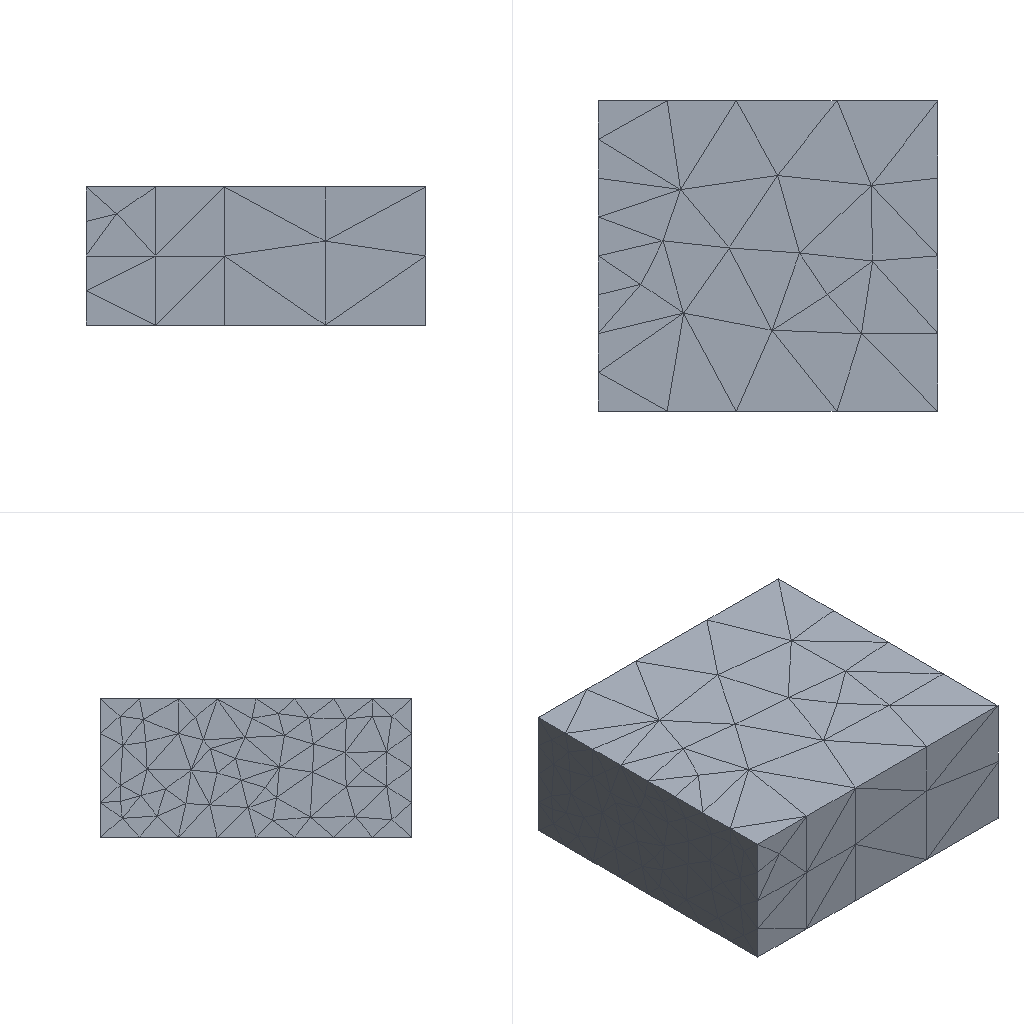Simulation study | ansys electronics desktop
Set-up summary:
category,name,step,type,value,unit,region
solver,ansys_electronics_desktop
units,length mm,,stated,model units
analysis,M06,,HFSS Modal Network,design_type=HFSS
setup,Setup1,M06,HfssDriven,frequency=10GHz; max_passes=2; max_delta_s=0.08
sweep,Sweep1_JEMY04,Setup1,Interpolating,8GHz..12GHz n=11 step=
sweep,Sweep1,Setup1,Interpolating,8GHz..12GHz n=11 step=
mesh,nodes,,,n/a (no mesh stored)
mesh,elements,,,n/a (no mesh stored)
material,vacuum,,permittivity,1
load,P1,M06,wave port,,,objects 34
bc,PerfE_TS6BF4,M06,perfect e,,,objects 58
bc,PerfE_YJ758H,M06,perfect e,,,objects 70
bc,PerfE_3KWRQP,M06,perfect e,,,objects 82
bc,PerfE_SXRUMP,M06,perfect e,,,objects 94
bc,PerfE_P8L5D8,M06,perfect e,,,objects 46
Ansys Electronics Desktop project file, long lists of numbers shortened, first 527 of 3724 lines:
$begin 'AnsoftProject'
	Created='Wed Sep 30 18:28:40 2026'
	Product='ElectronicsDesktop'
	FileOwnedByWorkbench=false
	$begin 'Desktop'
		Version(2026, 1)
		InfrastructureVersion(1, 0)
		$begin 'FactoryHeader'
			$begin 'geometry3deditor'
				KernelVersion(2, 0)
				ProjectContainsGeometry3D='1'
			$end 'geometry3deditor'
		$end 'FactoryHeader'
	$end 'Desktop'
	UsesAdvancedFeatures=false
	PreviewImageDesignId=1
	NextUniqueID=0
	MoveBackwards=false
	$begin 'HFSSEnvironment'
		Version(1, 0)
	$end 'HFSSEnvironment'
	$begin 'PlanarEMEnvironment'
		Version(1, 0)
	$end 'PlanarEMEnvironment'
	$begin 'Q3DEnvironment'
		Version(1, 0)
	$end 'Q3DEnvironment'
	$begin '2DExtractorEnvironment'
		Version(1, 0)
	$end '2DExtractorEnvironment'
	$begin 'NexximEnvironment'
		Version(1, 0)
	$end 'NexximEnvironment'
	$begin 'NexximNetlistEnvironment'
		Version(1, 0)
	$end 'NexximNetlistEnvironment'
	$begin 'EmitEnvironment'
		Version(1, 0)
	$end 'EmitEnvironment'
	$begin 'Maxwell3DEnvironment'
		Version(1, 0)
	$end 'Maxwell3DEnvironment'
	$begin 'Maxwell2DEnvironment'
		Version(1, 0)
	$end 'Maxwell2DEnvironment'
	$begin 'RMxprtEnvironment'
		Version(1, 0)
	$end 'RMxprtEnvironment'
	$begin 'MaxCirEnvironment'
		Version(1, 0)
	$end 'MaxCirEnvironment'
	$begin 'SimplorerEnvironment'
		Version(1, 0)
	$end 'SimplorerEnvironment'
	$begin 'IcepakEnvironment'
		Version(1, 0)
	$end 'IcepakEnvironment'
	$begin 'IcepakFEAEnvironment'
		Version(1, 0)
	$end 'IcepakFEAEnvironment'
	$begin 'SchematicEnvironment'
		Version(1, 0)
	$end 'SchematicEnvironment'
	$begin 'geometry3deditor'
		Version(1, 0)
	$end 'geometry3deditor'
	ReadVersion=12
	$begin 'DesignMgrEnvironment'
		CompInstCounter=1
		GPortCounter=0
		NetCounter=0
		Alias('Ieee;Simplorer Elements\\Ieee', 'Std;Simplorer Elements\\Std', 'Basic_VHDLAMS;Simplorer Elements\\Basic Elements VHDLAMS\\Basic Elements VHDLAMS', 'Digital_Elements;Simplorer Elements\\Digital Elements\\Digital Elements', 'Transformations;Simplorer Elements\\Tools\\Transformations\\Transformations', 'HEV_VHDLAMS;Simplorer Elements\\HEV VHDLAMS\\HEV VHDLAMS', 'automotive_vda;Simplorer Elem
	$end 'DesignMgrEnvironment'
	$begin 'ProjectDatasets'
		NextUniqueID=0
		MoveBackwards=false
		DatasetType='ProjectDatasetType'
		$begin 'DatasetDefinitions'
		$end 'DatasetDefinitions'
	$end 'ProjectDatasets'
	VariableOrders[0:]
	$begin 'Definitions'
		$begin 'Materials'
			$begin 'vacuum'
				CoordinateSystemType='Cartesian'
				BulkOrSurfaceType=1
				$begin 'PhysicsTypes'
					set('Electromagnetic')
				$end 'PhysicsTypes'
				$begin 'AttachedData'
					$begin 'MatAppearanceData'
						property_data='appearance_data'
						Red=230
						Green=230
						Blue=230
						Transparency=0.95
					$end 'MatAppearanceData'
				$end 'AttachedData'
				permittivity='1'
				ModTime=1499970477
				Library='Materials'
				LibLocation='SysLibrary'
				ModSinceLib=false
			$end 'vacuum'
		$end 'Materials'
		$begin 'SurfaceMaterials'
		$end 'SurfaceMaterials'
		$begin 'Scripts'
		$end 'Scripts'
		$begin 'AnsysComponents'
			NextUniqueID=0
			MoveBackwards=false
			$begin 'AnsysComponentDefinitions'
			$end 'AnsysComponentDefinitions'
		$end 'AnsysComponents'
		$begin 'Symbols'
			$begin 'M06'
				ModTime=1790764121
				Library=''
				ModSinceLib=false
				LibLocation='Project'
				HighestLevel=1
				Normalize=true
				InitialLevels(0, 1)
				$begin 'Graphics'
					Rect(0, 0, 0, 0, 0.00254, 0.00254, 0.00508, 0.00508, 0, 0, 0)
					Rect(0, 1, 0, 0, 0.0004233, 0.00254, 0.0004233, 0.0004233, 0, 0, 0)
				$end 'Graphics'
			$end 'M06'
		$end 'Symbols'
		$begin 'DefInfo'
			M06(1002, 0, 0, 0, '', 1790764121, '', 'M06', '', '', '', '', '', 'Design.bmp', '', 'Project', '', '', 1790764121, '', 0, 0)
		$end 'DefInfo'
		$begin 'Compdefs'
			$begin 'M06'
				Library=''
				CircuitEnv=0
				Refbase='U'
				NumParts=1
				ModSinceLib=true
				$begin 'Properties'
					TextProp('Representation', 'SRD', '', 'M06')
					TextProp('Owner', 'SRD', '', 'HFSS')
				$end 'Properties'
				CompExtID=6
				$begin 'Parameters'
					ButtonProp('CosimDefinition', 'D', '', 'Edit', 'Edit', 40501, ButtonPropClientData())
					MenuProp('CoSimulator', 'D', '', 'DefaultNetlist', 0)
				$end 'Parameters'
				$begin 'CosimDefinitions'
					$begin 'CosimDefinition'
						CosimulatorType=4
						CosimDefName='DefaultNetlist'
						IsDefinition=true
						Connect=true
						Data()
						GRef()
					$end 'CosimDefinition'
					DefaultCosim='DefaultNetlist'
				$end 'CosimDefinitions'
			$end 'M06'
		$end 'Compdefs'
	$end 'Definitions'
	DesignIDServer=2
	MoveBackwards=false
	$begin 'HFSSModel'
		RepRewriteV2=true
		Name='M06'
		DesignID=0
		'Use Advanced DC Extrapolation'=false
		'Use Power S'=false
		'Export FRTM After Simulation'=false
		'Export Rays After Simulation'=false
		'Export After Simulation'=false
		'Allow Material Override'=false
		'Calculate Lossy Dielectrics'=false
		'Perform Minimal validation'=false
		$begin 'TemperatureSettings'
			IncludeTemperatureDependence=false
			EnableFeedback=false
			Temperatures(6, '22cel', 34, '22cel', 46, '22cel', 58, '22cel', 70, '22cel', 82, '22cel', 94, '22cel')
		$end 'TemperatureSettings'
		ObjsEnabledForDeformation()
		'Port Validation Settings'='Standard'
		'Save Adaptive support files'=false
		SolutionType='HFSS Modal Network'
		$begin 'DrivenOptions'
			AutoOpen=false
		$end 'DrivenOptions'
		HasTransientSetups=false
		MaterialDensity=1
		MassOfTissue=1
		VoxelSize=1
		TissueObjectList=-1
		AverageSarMethod=0
		UseAutoDCThickness=true
		HaveZwaveSupport=true
		SolveInsideThreshold=100000
		RequireBodyFaceInfo=false
		$begin 'OutputVariable'
			NextUniqueID=0
			MoveBackwards=false
		$end 'OutputVariable'
		$begin 'ModelSetup'
			$begin 'DesignDatasets'
				NextUniqueID=0
				MoveBackwards=false
				DatasetType='DesignDatasetType'
				$begin 'DatasetDefinitions'
				$end 'DatasetDefinitions'
			$end 'DesignDatasets'
			VariableOrders[0:]
			$begin 'Editor3D Doc Preferences'
				BackgroundColorVersion=1
				'Plane Background'=0
				'Need Lights'=true
				'Ambient Light'=8355711
				'Num Lights'=1
				Light0[4: 16777215, 0.75, -0.15, -0.63]
				Ver=2
			$end 'Editor3D Doc Preferences'
			SnapMode=31
			WorkingCS=1
			$begin 'GeometryCore'
				BlockVersionID=3
				DataVersion=2
				NativeKernel='PARASOLID'
				NativeKernelVersionID=26
				Units='mm'
				ModelExtents=10000
				InstanceID=-1
				$begin 'ValidationOptions'
					EntityCheckLevel='Strict'
					IgnoreUnclassifiedObjects=false
					SkipIntersectionChecks=false
				$end 'ValidationOptions'
				ContainsGeomLinkUDM=false
				$begin 'GeometryOperations'
					BlockVersionID=2
					$begin 'AnsoftRangedIDServerManager'
						$begin 'AnsoftRangedIDServer'
							IDServerObjectTypeID=0
							IDServerRangeMin=0
							IDServerRangeMax=2146483647
							NextUniqueID=105
							MoveBackwards=false
						$end 'AnsoftRangedIDServer'
						$begin 'AnsoftRangedIDServer'
							IDServerObjectTypeID=1
							IDServerRangeMin=2146483648
							IDServerRangeMax=2146485547
							NextUniqueID=2146483654
							MoveBackwards=false
						$end 'AnsoftRangedIDServer'
					$end 'AnsoftRangedIDServerManager'
					StartBackGroundFaceID=2146483648
					$begin 'CoordinateSystems'
					$end 'CoordinateSystems'
					$begin 'OperandCSs'
					$end 'OperandCSs'
					$begin 'SubModelDefinitions'
					$end 'SubModelDefinitions'
					$begin 'Groups'
					$end 'Groups'
					$begin 'UserDefinedModels'
					$end 'UserDefinedModels'
					$begin 'OperandUserDefinedModels'
					$end 'OperandUserDefinedModels'
					$begin 'ToplevelParts'
						$begin 'GeometryPart'
							$begin 'Attributes'
								Name='Cav'
								Flags=''
								Color='(230 230 230)'
								Transparency=0.8
								PartCoordinateSystem=1
								UDMId=-1
								GroupId=-1
								MaterialValue='"vacuum"'
								SurfaceMaterialValue='""'
								SolveInside=true
								ShellElement=false
								ShellElementThickness='0mm'
								ReferenceTemperature='20cel'
								IsMaterialEditable=true
								IsSurfaceMaterialEditable=true
								UseMaterialAppearance=false
								IsLightweight=false
								IsAlwaysHidden=false
							$end 'Attributes'
							$begin 'PhysicsAttributes'
								SuppressedForPhysics='False'
								SuppressedForPhysicsEditable=true
							$end 'PhysicsAttributes'
							$begin 'Operations'
								$begin 'Operation'
									OperationType='Box'
									ID=5
									ReferenceCoordSystemID=1
									$begin 'BoxParameters'
										KernelVersion=23
										XPosition='0mm'
										YPosition='0mm'
										ZPosition='0mm'
										XSize='25mm'
										YSize='22.86mm'
										ZSize='10.16mm'
									$end 'BoxParameters'
									ParentPartID=6
									ReferenceUDMID=-1
									IsSuppressed=false
									$begin 'OperationIdentity'
										$begin 'Topology'
											NumLumps=1
											NumShells=1
											NumFaces=6
											NumWires=0
											NumLoops=6
											NumCoedges=24
											NumEdges=12
											NumVertices=8
										$end 'Topology'
										BodyID=6
										StartFaceID=7
										StartEdgeID=13
										StartVertexID=25
										NumNewFaces=6
										NumNewEdges=12
										NumNewVertices=8
										FaceNameAndIDMap()
										EdgeNameAndIDMap()
										VertexNameAndIDMap()
									$end 'OperationIdentity'
								$end 'Operation'
							$end 'Operations'
							$begin 'SubregionDependencyInformation'
								ChildSubregions[0:]
							$end 'SubregionDependencyInformation'
						$end 'GeometryPart'
						$begin 'GeometryPart'
							$begin 'Attributes'
								Name='Port1'
								Flags=''
								Color='(230 230 230)'
								Transparency=0.8
								PartCoordinateSystem=1
								UDMId=-1
								GroupId=-1
								MaterialValue='"vacuum"'
								SurfaceMaterialValue='""'
								SolveInside=true
								ShellElement=false
								ShellElementThickness='0mm'
								ReferenceTemperature='20cel'
								IsMaterialEditable=true
								IsSurfaceMaterialEditable=true
								UseMaterialAppearance=false
								IsLightweight=false
								IsAlwaysHidden=false
							$end 'Attributes'
							$begin 'PhysicsAttributes'
								SuppressedForPhysics='False'
								SuppressedForPhysicsEditable=true
							$end 'PhysicsAttributes'
							$begin 'Operations'
								$begin 'Operation'
									OperationType='Rectangle'
									ID=33
									ReferenceCoordSystemID=1
									$begin 'RectangleParameters'
										KernelVersion=23
										XStart='0mm'
										YStart='0mm'
										ZStart='0mm'
										Width='22.86mm'
										Height='10.16mm'
										WhichAxis='X'
									$end 'RectangleParameters'
									ParentPartID=34
									ReferenceUDMID=-1
									IsSuppressed=false
									$begin 'OperationIdentity'
										$begin 'Topology'
											NumLumps=1
											NumShells=1
											NumFaces=0
											NumWires=1
											NumLoops=0
											NumCoedges=0
											NumEdges=4
											NumVertices=4
										$end 'Topology'
										BodyID=34
										StartFaceID=-1
										StartEdgeID=35
										StartVertexID=39
										NumNewFaces=0
										NumNewEdges=4
										NumNewVertices=4
										FaceNameAndIDMap()
										EdgeNameAndIDMap()
										VertexNameAndIDMap()
									$end 'OperationIdentity'
								$end 'Operation'
								$begin 'Operation'
									OperationType='CoverLines'
									ID=43
									$begin 'LocalOperationParameters'
										KernelVersion=23
										LocalOpPart=34
									$end 'LocalOperationParameters'
									ParentPartID=34
									ReferenceUDMID=-1
									IsSuppressed=false
									$begin 'OperationIdentity'
										$begin 'Topology'
											NumLumps=1
											NumShells=1
											NumFaces=1
											NumWires=0
											NumLoops=1
											NumCoedges=4
											NumEdges=4
											NumVertices=4
										$end 'Topology'
										BodyID=-1
										StartFaceID=44
										StartEdgeID=-1
										StartVertexID=-1
										NumNewFaces=1
										NumNewEdges=0
										NumNewVertices=0
										FaceNameAndIDMap()
										EdgeNameAndIDMap()
										VertexNameAndIDMap()
										$begin 'GeomTopolBasedOperationIdentityHelper'
											$begin 'NewFaces'
												$begin 'Face'
													NormalizedSerialNum=0
													ID=44
													$begin 'FaceGeomTopol'
														FaceTopol(1, 4, 4, 4)
														$begin 'FaceGeometry'
															Area=232.258
															FcUVMid(1.51681195174844e-15, 11.43, 5.08)
															$begin 'FcTolVts'
																TolVt(0, 0, 0, 5e-07)
																TolVt(1.39977129142543e-15, 22.86, 5.07593966858622e-15, 5e-07)
																TolVt(3.03362390349689e-15, 22.86, 10.16, 5e-07)
																TolVt(1.63385261207146e-15, -2.25597318603832e-15, 10.16, 5e-07)
															$end 'FcTolVts'
														$end 'FaceGeometry'
													$end 'FaceGeomTopol'
												$end 'Face'
											$end 'NewFaces'
											$begin 'NewEdges'
											$end 'NewEdges'
											$begin 'NewVertices'
											$end 'NewVertices'
										$end 'GeomTopolBasedOperationIdentityHelper'
									$end 'OperationIdentity'
									ParentOperationID=33
								$end 'Operation'
							$end 'Operations'
							$begin 'SubregionDependencyInformation'
								ChildSubregions[0:]
							$end 'SubregionDependencyInformation'
						$end 'GeometryPart'
						$begin 'GeometryPart'
							$begin 'Attributes'
								Name='Short'
								Flags=''
								Color='(230 230 230)'
								Transparency=0.8
								PartCoordinateSystem=1
								UDMId=-1
								GroupId=-1
								MaterialValue='"vacuum"'
								SurfaceMaterialValue='""'
								SolveInside=true
								ShellElement=false
								ShellElementThickness='0mm'
								ReferenceTemperature='20cel'
								IsMaterialEditable=true
								IsSurfaceMaterialEditable=true
								UseMaterialAppearance=false
								IsLightweight=false
								IsAlwaysHidden=false
							$end 'Attributes'
							$begin 'PhysicsAttributes'
								SuppressedForPhysics='False'
								SuppressedForPhysicsEditable=true
							$end 'PhysicsAttributes'
							$begin 'Operations'
								$begin 'Operation'
									OperationType='Rectangle'
									ID=45
									ReferenceCoordSystemID=1
									$begin 'RectangleParameters'
										KernelVersion=23
										XStart='25mm'
										YStart='0mm'
										ZStart='0mm'
										Width='22.86mm'
										Height='10.16mm'
										WhichAxis='X'
									$end 'RectangleParameters'
									ParentPartID=46
									ReferenceUDMID=-1
									IsSuppressed=false
									$begin 'OperationIdentity'
										$begin 'Topology'
											NumLumps=1
											NumShells=1
											NumFaces=0
											NumWires=1
											NumLoops=0
											NumCoedges=0
											NumEdges=4
											NumVertices=4
										$end 'Topology'
										BodyID=46
										StartFaceID=-1
										StartEdgeID=47
										StartVertexID=51
										NumNewFaces=0
										NumNewEdges=4
Last 209 lines:
3eHl6goOEhYaHiImKkpOUlZaXmJmaoqOkpaanqKmqsrO0tba3uLm6wsPExcbHyMnK0tPU1dbX2Nna4u\
Pk5ebn6Onq8vP09fb3+Pn6/9oADAMBAAIRAxEAPwD+/iiiigAooooAKKKKACiis7WNY0jw7pGq+IPEG\
q6boWg6Fpt9rGt63rF9a6ZpGj6RplrLe6lquq6leypDp+m29nBNNPPM6RRRQtJIyopIANGiviP9mX4v\
/E74pfGL44y+MrnUtJ8D3/w8/Z/+JPwu+F+t6DpWleIvhXpHju5+Mfh/UtE8U39vpNve33i6/X4caRq\
urWd5LdRaFqWr3WhafdXtpp66pqP25QAUUUUAFFFFABRRRQAUV/Lb+0J/wXq+Mnwp/be8d+APCXwv+F\
+vfsRfBn9oL4cfAf4u/F+88O+OL7xtpOqa2mpweN5LDxFpvj6DR7fUIr3wZ8Tn0iGTSLhLq28Eu0jkz\
Ap/Ttrfijw14a8Nav408R+ItC0DwdoGhX/ijXvFmt6tYaV4a0Tw1pVhLquqeItX12/uI7XTdCttLgnu\
bi7mlS3ht4XmkkWNSwANyivna6/a/wD2S7LQPCHiu9/ai/Z2tPC/xBN8PAXiS6+Nnw1t9A8bnS9YvfD\
2pjwhrEviYW/iU2+v6dqFjP8AYpJvJvLCa2k2zROi+63uuaJpujXHiPUdY0qw8PWenvq93r17qFpa6N\
a6VHAbqTU7jVJ5lgg09bYGRpmkEYjG8tt5oA1KK8L+Hv7UP7M/xb8QzeEvhT+0T8C/ib4rt455Z/DPw\
9+LfgDxp4hgitVZ7qSbRfDfiC5uY440VjIWiAQKSxAFdd4L+MPwj+JGveOfCvw7+KXw58e+J/hjrJ8O\
/Erw54L8b+GfFOvfD3xALzVNPOheOdH0PU57jwnrP2/Q9ag+y38dvP52j3UWzfbyqgB6NRXnOpfGH4S\
aN8SfD3wa1j4pfDnSfi/4t0m41/wp8KdS8b+GbH4k+J9Cs4dYubvWvD3ga61NNU1rSYrfw74gkkuba1\
lhRNCvHZwtrOU4LU/2tv2VNF8Zv8ONZ/aa/Z80n4hRX50uXwHqfxn+HFh4zj1MS+QdOfwvdeJEvkv/A\
Dvk8kwCTd8u3PFAH0HRR16UUAFFFFABRRRQAUUUUAFfFXx98Vt8R/F7/A3SpZD4O8Lx6Pr3xzmWWK40\
nxfaeItI8Qr4f+BF0LLLpJKP7A8S+KrS4uLXfoFz4e0e803XPD/jnUhZfQPxi+KFt8J/B668ul/8JH4\
i1nXNE8IeCPCUeox6bceKPF3iO8W0sbQ3Itrme30OxsV1LWteu7Sx1G60rw34X1nWU069TTpLd/kbwX\
4au/DWirHresyeK/GeryQ6z8QPHN1aCx1Hx542m0+xstZ8VX9oLmYadHKlhawWOnRStZaLpWn2Gh6Wl\
vpOm2NrAAdb+z1/ycl8fP8Ash/7Mf8A6nv7WFfcFfD/AOz1/wAnJfHz/sh/7Mf/AKnv7WFfcFABRRRQ\
AUUUUAFfIX7ev7TFj+yB+yF8dv2gZ5rdNX8D+CL5PBVtchHj1H4ieIpIfDXgCweB8m4t38W6vpDXKqr\
FLSKeUqUjYj69r84P+Ckf7AWpf8FD/Afwq+FGofG25+E/wz8HfE6x+IvxC8P6f4EfxXqPxMi0q0k03S\
9Ah1tfHGkjwnDDYap4jPnNbaorXOoWl19nD2CLMAfxofCb9tf9h7QP+CW/x4/Y/wDiZ4K/aA8Q/tJ/H\
PxZr/xb1b4n6f4R+HmqeErP4raLqdndfC1/+En1b4r22sSeH0tNCsk1af8Ask3EZ8Y68Le2uxKpuP6H\
/wBk/wDan/4al/4IBftD3mr6l9v8e/Bf9jz9pr4FePTLL5l3Jd+AvgX4mi8Japcs58y4kvfh9e+FJpr\
hx++vfto3u0bmv6IdM0zT9F03T9H0myttO0rSbG00zTNPs4kgtLDT7C3jtbKytYIwFhtoraKNERQAqx\
gAYFfj/wDDz/gkt/wqvVP+Ckem+Bvj/wD2T8Jv+ChPgT4leHv+FXt8KvOg+C3i74haP4t0mPxdo2tp8\
SI4/FGm2K+O/E4GlJp+j/abc2Fs1/ELBJJAD8Jf2XP+CV37L/xT/wCCJfxH/bI+IGm+Ldf+O9t8Gf2m\
fib4A8Snxr4kstN+H0HwO134nJo3hbRfCtlqCaXeaLf6n4G1C5v/ALdaXUzSeJ7p7aW2k2SL9QeHf2f\
P2nf26v8Ag3T/AGZPh78Dtaude+IuleJ9e1HU/Cd/4jt9Fm+JPw4+F3xk+NXg3SPh3Fq2s3kFmi2UNr\
4LvbOC9uILU/8ACDW8CyI4gFfqx4S/Zs+Cv7Hn/BNyP/gnB8WP2u/hd4TvfiF8J/2h/g94X+KnxEfwn\
8MrrW7r46az8Rr99V0H4b+JfiUX1640iX4lwRGyt9aZr1tNQm4szdBYfPof+Cff7I3hL9gX4T/8En/2\
j/2j/A+v6/JdeJta+GHiCbWPB/wm+KWs+LvEXxQ8deO/D/ij4c/DrXvGGrT3t9ZTeMdQ0loopdRi1C3\
S7jdYhdNDCAfgPN8X/gP4K+IX7OXhf9u3/gnX8Tf+CafxO+FPxB8O6j4R/ah/Y68MaN8H/wC1tV014L\
ZLvxZoPj3wBqVv438IQ3cdtfX1/Z6vrmohLSVbQvDLdWt5+qPxN1GD/gnT/wAF0PBnxKup4vD37Pf/A\
AUm8Fjwj4vuriRLLw/pHxj0y40zSv7ScyssUd3/AMJhB4Iurq7mkVYovi3qspwqkHvJf+Cd+lfGn4rf\
Cj9nT9sn/grHb/tZ6H8C/EekeOPCv7IE/h34MfDv4kX154X0eePSpviLPonjPUPE3jS1Xw7d3kd5c3l\
kt7NY6jdGO9tTcSTV8Cf8F2f28v2O/wBrL4Tan+zn8OtUvPiB+0N8Jv2lfDNh8KbzwLpOva5pfiLw9f\
eAdIXxXr9t4kl8O29jfaFf+IfE2qaJZ2OkXmqy6ne+C9N1m3kbTbuBgAe/fsOeE/Gn/BST9qX/AIKc/\
t8+GvEM/hiK88C/ED9j/wDYw8bXBu4rfwZeal4LudF03x/pbQIZtI1Ow0IeENTm8jewn+JuqBAXAJ/K\
hfh34x/Ym+Bni79m/wD4KF/8ElIPGHw/urjX0uv2z/hJo+lwfGnwyusatcala+JdL+Pi+H/Emiale2U\
k0Q0zT7u50a3a0t4rXVbO5Auo5v6jv2Vfh3+zB/wT1/YH+Bf7L/7UnxO+CHwpn+IHw38Rn4i6L8Y/iP\
4J8A23xC8XeNbO31L4y6LaSeKtcsv+EostOl8Z2mjzPblzDYLp6S+UJYQfjfw1/wAEs9Rs/wBnvx18P\
P2cP+Cs3iDwt/wTi8dWfjrVNc8C2fgv4PfFDw9YfD7W5NRn+IWk6J+0dL4qj/sLwmYP7ZXUJIIo7bD3\
cuoLPLLeSTAH6tf8E7vFHwq8ZfsUfs7678EPHPxR+I3wpfwINK8F+KfjVc6LefFRtL8Oa1q3hyTw942\
uvDumWljPrOi32k3eilrWFojH4fj23F5zdzlen/sqfCT4OfAv9nP4O/C39n2+s9Y+DPhnwRpUnw+8RW\
GuWHie08W6F4gWTxMPG0XiTST9k1863d6zdas17ZhbO5fWWmtES3eNFKAPoGiiigAooooAKKKKAPg74\
rX13r/7T+p+HtYnkv8AQvhx8GfhZ418FaTMR9g0Lxh8SPFnx/8ACni/xRDbIAt14gn8L+B9D063u7gT\
T6bY3OqWumPZwa7riajo1h+P/wDk7f4lf9m5/s5f+rM/aurcoAP2ev8Ak5L4+f8AZD/2Y/8A1Pf2sK+\
4K+H/ANnr/k5L4+f9kP8A2Y//AFPf2sK+4KACiiigAooooAKKKKACiiigD8cv+Cp+p6T4w/4Rz9k/4M\
fCPwD49/bR/bK+HnjD4J6T481rwpo15qnwY/Zjv50X4u/EPxZ4x/s9tQ0fwTZ/2jJ/ZtilxFHd65MLm\
0iur6yW0ufxc/bJ+H3/AAqS1/4Ky/CuXWrzxL8Rfhn8Pf8Agiv8P/2afEfiQwt478QQ+DJ/B3hvVtb8\
OsSZW1K78RaZq09+bMkG6nm3EnNf1d/FH9lz9mb44a5ZeJ/jT+zr8Cvi/wCJdN0mLQdO8Q/FH4R/D/x\
/rmn6HBeXuoQaLZat4s8P3dxa6Sl/qWozpbRyLCs1/PKEDyyM2V40+E37LHgKx8JfE/xj8HfgxpX/AA\
o7QNA8NfDXxM/wp8KX/iD4c6Jps9po/gzwV8KU07w3NqOkyHUbjTdP0LQ9AjFxc3t7a6dpVlLdzwQOA\
fiB+1ZdeHf2pv2/fh9+y1+zL4C0j4e+Bv2XPj1pn7U37Zn7QPwz0O38Fa3qnxum8L6vZ6X4Gj8aeDrr\
Sb2fxlqmj382nazqsWoS635+pmeJCfC14T4j+zn4D/Z+/wCHwfwQ8Q/Crwr8DvEvwsv/ABB+0tb/AAr\
H7Pfh/wAA6VYeAPGfgX9lz9nK78VeLviVrHhCyubbxn4LbVfEGuaboFnG2nroXi++1S9VpL6e8WX9Kv\
A37LPwQ1DX7n45/EL9nD4I2/x88c+P9Q+NniHxBc/DL4bap4t8EeONc1pPEWj6RpnjHTtEIn1zw5BDo\
tg+vacbSTXNV0G58V3CDWNYv7iX6P8A2LPhd8M/C/jv9rjxj4Z+HXgTw74u1X4+afpOqeKtC8I+H9I8\
R6lpVx+zz+zz4mn0y/1zT9PjurzT38Savq2oPDJK0bX2qXF2ym4nlkYA+R/+Ciep/EPRv+Clf/BH/U/\
hT4P8LePvH9nb/wDBQ2Xw94P8aeOtQ+GvhzXJP+Ge/Bq39rfeNtL8DeJJtEnXSWv5bU/2NdRXF3BBaz\
y2ME8t/a/E/wAO/g74I+Mn/BIX/gojrvjzV/EWk+OtH+M/7f37TfxN+BPh3WtY8I6Z8D/jzo/wz8dQ6\
f8AAfxZZ6dcRf8ACX+C9A1NdA8SWtuVh02+1SDTb17d0tXgk/pe1n4e+AfEfizwX498Q+B/B+veOvhv\
/wAJH/wrvxprPhnRdU8WeAv+Ew02LRvFv/CF+I76ykvPC39qaPBBaaj9hmg+3W0KQXPmxKEGFH8Ffg3\
CvxOSH4S/DKJPjZFcW/xmSPwH4VRfi5BeaXeaJdw/E5V0oDx7FLouoX9pIuq/aw9rfTW7AxSujAHhv/\
BPb/kwX9h7/s0D9mn/ANUx4Kor6n8PeHtA8I6BofhTwpoej+GPC3hjR9M8PeGvDXh7TLLRdA8PaBotl\
BpujaHoejabBFb6To9pp1tbW9tbW8ccMENukUSJGiqCgDYooooAKKKKACiiigD4D8f/APJ2/wASv+zc\
/wBnL/1Zn7V1blYfj/8A5O3+JX/Zuf7OX/qzP2rq3KAD9nr/AJOS+Pn/AGQ/9mP/ANT39rCvuCvh/wD\
Z6/5OS+Pn/ZD/ANmP/wBT39rCvuCgAooooAKKKKACiiigAooooAK+HPjjrd34z+Oun/C+/eRfBnwz+H\
ng34s6hobyCbTvGXjbx1428Y6V4A1TVLdEjKx+En+DviK9s7a4e9srvVfG+n6x9ls9W8KaPen7jr4D8\
f8A/J2/xK/7Nz/Zy/8AVmftXUAblbn7JP8AyGP2qf8As4zSf/WXf2aaw63P2Sf+Qx+1T/2cZpP/AKy7\
+zTQB9iUUUUAFFFFABRRRQAUUUUAFFFFAHwH4/8A+Tt/iV/2bn+zl/6sz9q6tysPx/8A8nb/ABK/7Nz\
/AGcv/VmftXVx3xU8b6h4N0XRrbw9BY3njPxt4o0vwV4MtdTjuZdNXVb+C+1jWta1GK3uLcXljovgjQ\
/FmvTWTXunvqsfhdtJtL+2v7+0egDB+GX7Qfwz+Hv7Tf7Qlp4gk8e3c1n8MP2c/Cl6fB3wd+MPxGhsf\
EGl6r8efGV5pt9dfDzwHqkVlKPDXxG8HXSNK6RzDVmiheSa1vI7f7N0L9qv9mjxHqWjaDpfx7+Eg8U6\
9fadpGneCNU8e+G9B+IA8QapcQ2Vp4V1H4f67qFtrWjeMf7RnjtJtGvLC31S3vd1lcWkV2jwr8IfBjw\
tYeCvFvibwvp1xfX0GkfDP4VQz6tq0sNzrmv6lN4m+Md3rHibxHfQW8Q1XxRqer3F9qGp3pjWS91DUr\
m7lBlmcn3/AFPTNN1vTdR0bWdOsdX0fV7G70zVtJ1O0t7/AE3U9Nv7eS0vtO1Gxu43ivbGa1lljmhkR\
o5I5WR1ZWIIB93UV+Xtl8A/hVofm/8ACEeHb74Tfatn9qf8KN8W+M/gP/b/AJG/7F/wlH/CmvEGhf8A\
CVfZfOu/sX9pfavsP9pXf2PyPtl153R23hz4naNAmm+E/wBpf47+GvD9tu+waJc3Pwp+JE9l5ztPdb/\
Gnxq+FPifxNrPmXstzMP7T1y++zicWln9m0+C0s7cA/R+ivg6z+LP7VOhStd3/wDwz78U4ZIzbL4fs9\
B+I3wDls5XZZV1lvGE3iv4kjUo40heA6Z/YVoZjqIuv7WgFmbO/wCjs/2o/iNpUTW/jP8AZn8Xanqjy\
Ga3n+CvxI+GPjjwslgyqkUN/q3xd1z4d6lb+IBcR3TS28GiXViltJaSxapPcTXNpYgH2dRXy9bftk/s\
+vOi6v4l8Y+CNPO77R4n+KPwZ+Nfwl8C6ZhGMX9ufEH4nfDzSND8P+dOIre2+3ahb/a7y7t7G2828ub\
eCX1vwB8YfhH8WP7W/wCFWfFL4c/Ev+wPsH9u/wDCAeN/DPjL+xf7V+2/2Z/a3/CO6nc/2b9p/s3UfI\
87Z532Cby93lPtAPRqKKKACvgPx/8A8nb/ABK/7Nz/AGcv/VmftXV9+V8B+P8A/k7f4lf9m5/s5f8Aq\
zP2rqANytz9kn/kMftU/wDZxmk/+su/s01h1ufsk/8AIY/ap/7OM0n/ANZd/ZpoA+xKKKKACiiigAoo\
ooAKKKKACiiigD4D8f8A/J2/xK/7Nz/Zy/8AVmftXV87+BL4/EbU5vjdd82ninRV0f4ZWGWmtNL+Fia\
zqOp6L4oszefvrHXPGNlJoOt6rGItPeOysPDeiajYNqHhyW/vN79p7Sdb8X/tc+KfAf2PyvAOvfs5/s\
/av8QNaS5t3lvrLwv8ZP2hbzTvhm+kzTr9q0XxN9r1GLWpZob2zl0HQdV0O4tFl161v7DtqAMfwT/yV\
Tx//wBk/wDhX/6kfxgr2ivF/BP/ACVTx/8A9k/+Ff8A6kfxgr2igAooooAKKKKACuH8Z/DH4bfEb+zf\
+FhfD3wP48/sb7Z/ZH/CZ+E9B8Uf2V/aP2X+0P7N/tzT5/sPn/YbLzvK2+b9ji37vLTHcUUAeV2vwk0\
nR/s7eEvG3xp8EtpXkt4ZsvDHx0+LsHhHwi1jtOjWvh74X6n4yuvCUPhywMVslpoFxoNx4dW2tI9Ol0\
ibTA1m3VWWr/tKeG/N/wCEf/aAsfGH23Z9r/4Xl8IfCPir+zvs+/7P/wAIv/wpG++G32DzvPm+2/2n/\
bPm/ZbT7F/Z3l3f27qqKAILb45/tOaTAmn3nw1+BHj+5t93meLrb4pfED4QQat5rtOmz4dS/Cfxw3h7\
yI5FtTnxRqn2s2Rvh9iFyNOtPlrxX+0ppD/tN+P/ABD4v+Fvxk+H1je/An4GaNFDqXhbRPiFqaXek/E\
D9o6+gluNJ+BHinxfcW9hew63ei2uHjEMUnhq8iv3sXuNIXVPqyvjPxr/AMnJeO/+yH/A/wD9T39oug\
D1O1/af+AMkZOr/FHw14GuQ5CaT8VJLz4Q+IbiDapXUbPw18UbTR9QvtGeQyxR30Ns9nLPaXFvHO09t\
cRxfSv7JP8AyGP2qf8As4zSf/WXf2aa+B/FvinTvBug3Wv6nHd3EMNzpenWtlYRxS3+qaxr2rWOgaBo\
9kLmeKCK7vdd1PTrWOW5nt7SF7xZbu5trZJZ4/oj/glzoE3hj4WfHHRbqz8Pade2/wC0G1zqOneEdKs\
NE8Kadqmp/AD4Aapqlh4a0zT9NtFg0CDUL25is2mhN7LbxRzahPdX0lzczAH6aUUUUAFFFFABRRRQAU\
UUUAFcR8RvH+i/DLwjf+L9dg1K9tre/wDD+iadpWjwW8+r6/4n8YeI9J8HeDfDGlC+u7a0t9S1Txdr2\
iadBPf3dlpttLqa3GpX1jYRXF3D29fIUeoD4u/Fy48dxM0/w5+EDeL/AIfeAYrgNENY+Llp4k1rwX8Z\
vG02jXTSiJdCHhv/AIRLw5qezTdSU6v8QoxDfeHdb0bUb0A+UNO8Iaz4S+JXiR/F9zp+pfEbxb8OPh5\
45+KGs6XNdXmnaj4/8T+NfjRea1a6LqGp20V9eeDNIhWx0Dwwmo+Ze2HhbwlomlSzSCwQ13lXviN/yX\
bxN/2SX4V/+pj8aqo0AY/gn/kqnj//ALJ/8K//AFI/jBXtFfNWiePvAnhn4sePofEnjXwl4fmPgf4Y2\
gi1vxHo+lSG7t9Y+KF/PbBL+8jJuEsdW0qZ0xuWLU7eRgEmjLfRlle2epWdpqOnXdtf6ff20F7Y31lP\
FdWd7Z3UST2t3aXUDslzbSQSI8ciMyOjhlJBBoAs0UUUAFFFFABRRRQAUUUUAFfGfjX/AJOS8d/9kP8\
Agf8A+p7+0XX2ZX5yfHzxRqWn/tJeJPCHhe6+yeMvF3wP+C1xZXzW9vLFoPhPQ/if8bLfxv4oV76KS3\
bVLXT9esrfS4ZIL5ZdY1rT3utPn0mHVJrYAwbq/wD+Fg+Mhq6nf4O+Huranp/hcbfstzqPxG0yTxX4I\
8da3cpzNLpOnWlzf6LpySG1Sa6n1y7ms722Xw9qSfon/wAE9f8AkWv2i/8As4xf/Wd/2ea+CdE0bTfD\
mi6R4e0a2+x6PoOl6fo2k2fnXFx9k03S7SKxsbb7RdyySz+XawRLvkd5G2bndmJJ+9v+Cev/ACLX7Rf\
/AGcYv/rO/wCzzQB+g1FFFABRRRQAUUUUAFFFc54x8W+H/APhHxT478W6h/ZPhXwV4c1zxb4m1X7Je3\
/9meH/AA5pl1rGs6h9h0y2mubzydNs7mTyreGWeTy9kUckhVSAeM/tB+JtUudL074L+DNV1LRviD8YN\
N1qCHXdKvLvRdQ8FfC7Q9V8J6P8X/iJo/iS2mR9G8ZaboPjbTLTww9ul9cr4q8UaHdz6bNoVnrt7p2z\
pOk6VoGlaZoWhaZp+i6Joun2Wk6No2k2Vtp2laTpWnW0dnp+maZp9nGkNhp8FpDDFDDEiRxRxKiKqqA\
PPfhtoXiA3njX4j+ObFtP8d/E3xFJql1pU91aahceDPAeiedpHwv+HUd3aXd3HZtp/hdBqWs2NnqWo6\
MnjXxt4u1HRbqSw1WNm9SoA+PfiN/yXbxN/wBkl+Ff/qY/GquT8Ra2dEsrd7e0/tHVdT1Gx0XRNKE5g\
bUNV1GYRRLJIkMskWnW1sLq+1CaGC5ktNN0u8vRbzLbNGes+I3/ACXbxN/2SX4V/wDqY/GquD8LQ/8A\
CU65d+MbhftGgaf5Fj8P9432d0rWU39uePNO5Tf9u/tKTTLKaSJ8WGiTXumXb6d4hm88A6vwr4eXw3o\
8FlNdDU9XnEd54i154Ps1z4j1+S2t4NQ1q6hM0n2cy/Z4kgt1kaGxtLe3sLQR2drbxR4938L/AIc3l5\
c6nL4G8Kxaxd3M1/Jr1loen6d4ij1OeVrh9XtPEWnwRX1hrQunM0d7BcR3UU4E8UyTKrju6KAOETwRd\
WGf+Ec8f/Efw75uPtm/xMPG/wBs8vP2fH/C1LHX/wCzPL3z/wDHh9k87z/9K8/yrfybCR/FTTNqWPjH\
wz4jsrU+bHB4t8IzWviLVgD50ljf+KfCuuWen6aZJC8MN1B4ak+ywGJ5bPUZopGuezooA5VPGvxCsT5\
us/DSwv7Vh5ccPgTx5Z67q63Bwyy3Np420HwzaR6aI0lDyR381wJXhVLSSN5ZrewnxX0y2Hl+IPCXxG\
8OXpO+KxfwRrHjAy2pwqXf9p/DGPXbCANKsyeRNdx3i+R5klskMtvLN0VFAEGj/E34beIdRt9H0D4g+\
B9c1a8877Jpej+LNB1PUbr7PBLdT/Z7Kyv3ln2W0E0j7VO2OFnbCqSO3rz7VtH0nXtPuNJ13S9O1rSr\
vyvtWmatZW2o6fc+RPHcwfaLO8ieObZcwwyJuU7XiVxhlBHIJ8L/AAZajy9GsdV8J2pO+TTvAnirxZ8\
P9ImuDhWvbnRvBOt2Fpc6k0axRvdSQtcPFbQxPK0cMSIAe4UV4uvhrxZZbTpPxU8ZxxWmDpml61YeCd\
f0mOOD/jzsNWurnwpHrWt6cFSOOeSTWk1S5iDs+qLdubsWU1X4u6bnzIvhx4z87GNjeJvhn/Zvl5znd\
/wlv9t+d5g/6B/2b7L/AMvX2j/RgD0PxP4k0Xwb4a8Q+L/El7/Zvh3wroereJNe1H7Pd3n2DRdDsLjU\
9UvfslhBLPdeVY2s7+XDFJK/l7Y43cqp/N+5v/GOr/Hb4ha143/0TU9Y+Gvwxv8ATfDqrpezwh4Xf4g\
/H+Hwr4bnm0oypda5HoMFjca1J9v1SA67qWqLpl++jLpsEHpvxK+LPiLxZ4qsfBerfDHxTf8Agv4ceI\
bPVfi7eeBr3w94js7fx34eb4d/E34Y2mmnUtT0zxF4m8OafpWq22v6rBo/h4andarpekaVp41a0Or6b\
f8AgniX4yfDt/jj4u1bU9Zv/CGmXPwo+FOnQX/xG8L+LPhjay31h4v+NVzNaJN8Q9D0wNcPb6nE9suc\
3i2d8bTzhp2ofZgD2KvuL/gnr/yLX7Rf/Zxi/wDrO/7PNfn/AOHvFPhjxdZS6l4U8R6D4n06C6exmv8\
Aw9q+n61ZQ3sUUE8lnLdabcSxx3SwXNs7Rlg4S4RiMOpP6Af8E9f+Ra/aL/7OMX/1nf8AZ5oA/Qaiii\
gAooooAKKKKACvkn9qvQNQ8Zaj+zJ4HtPF/iTwVaeK/wBosLqmq+GIPCt9fOvg/wCAnx4+JWgLJpPjr\
wxrWjamtt408EeF9Rtxf6VefY7/AESz1Ox+y6pY2F9a/W1fN/xz/wCSkfsf/wDZxnib/wBZJ/akoA5V\
/BX7VejqdRj8e/s+fEN7fG3we/wu+I/wbXWPOIgOfiQvxd8dnw59nEpuv+RU1X7YbL7B/oP2r+0rOjJ\
4w+PegMLPxP8Asza54mv5R9phv/gh8VPhd4v8KQ2bkxR2moal8adc+HGqQeIVmhuHlgt9DutPW2uLSS\
LVZ7iW6s7H64rH8QeINI8L6Re69r16thpdgsRnnMU9xLJLcTxWllZWVlaRST6lqlzfXFtbWlpbRy3V3\
dXUNtbQyzyxxsAfkN8ZPi1a33xf1K3vvDPxg8AWt14J+FmjfELV/EHwp+JWk2Pw60jQvE3xn1jxjca5\
460vw/Lodr4fKImkN4r0zXpNBt01S517SdfurPSJrpfVPAfj74X+MrSew+GPjTwD4rsPDVtptnc2XgP\
xH4e1208P2k0U8Oj2s9t4fvJU0q2eHTrlLZGWNWWxkWIERMF+gvD0er3i3XinxVC0fi/xSw1DWIJriC\
9l0Cxa5vLvQvAtte2jGCfS9DsdQayjktUht726W81hoFvdUvZJcfxt8LPhj8S/7M/4WN8OfAfj/wDsX\
7b/AGN/wm3hDw/4q/sn+0vsn9o/2Z/bunz/AGDz/sFj53lbPN+xRb93lptAOSorFm/Zj+FVuXk8JReM\
/hq8S+Zotj8NfiN478H+DfDN+i74dR0T4Uadr/8AwhysL8G8uLS68P3Wm6ldyzzatY6h9rvFuMub4J/\
E3SlFx4W/aF8R6tqDsIZrb4vfDz4c+LvDSWbAvJPY6b8KtG8BajBrgnjt1inm1i5slt5bmOTTZp5be6\
swDrqK4Gbwz+0rorC1gtPgb8SkkUXB12bXvH3wQa0ZyYzpI8KJ4Y+II1BYxEJv7R/tq1837ebb+y4fs\
n2u9ypPiB4z01GvfE/7Pvxt8NaHDj7drUdn8NPHz2XmERW2PCXwh+JviPxFq3mXklvCf7O0a88gT/ab\
v7PYw3N1AAep0V41N+0J8GdOYQeKfHuk/DjUHUSw6H8XoNT+DXiW6s2JSPVbHwx8VbHR9Rv9DedLiGK\
/htZLKW4sbm3jnae1uI4vWNN1LTta07T9Y0fULLVtI1aytdS0vVNNuoL/AE7UtOvoI7qx1DT761keK8\
spraWKSKWNmjkjkV0YqQSAXaKKKACvNfip42vPBnhuNNAhs7zx14tvLnwp8ONO1OG4k0a98az6DreuW\
UniGW3uYGtfDNlpeg6vqepsk6XT2GiXMGmpd6rNY2N16VXyp4e1P/hZfiAfF+U+ZoFzpE+lfBxQn2SV\
fht4ltfCms6p4l1azBaQav4h17QbC8hjuZS9noekaHE2n6NrEviG3uADo/DHhyz8K6OmkWc95eFr/Wt\
Z1HUdQe3a/wBY1/xNrWoeJPEuuXy2dtBbwXl94h1bVLyWG0t7ayge9aGytbW1SG3j+dvFf/JevGP/AG\
SL4Rf+pl8c6+qa+VvFf/JevGP/AGSL4Rf+pl8c6AOY8V+C/h5rs0Or+L/A/hnxTqKiw0XT5NS8H2Piv\
Xrya+1EWujeHdDs/wCy7m91XUrvWtTS3sNOs45bi7vdTS3tIJbm4SN/2U/Yw+At78Afg4mma9Lri+Nf\
iJrcfxQ8f6NrniGfxXJ4R8V614T8KeHpfBNl4kvNY1KfX7fSNG8K6NYTX8mo3UeoX1ld39iun6bdWWk\
6f8cfsjfBmX4q/EO2+Jmv2dx/wrX4S63bX3hWSWztLnRfiP8AFSxPiPSb2BxqO5bvRPBV/Fp18s9vbT\
I3jE2H2TVbDVPBer6fcfr3QAUUUUAFFFFABRRRQAV83/HP/kpH7H//AGcZ4m/9ZJ/akr6Qr5v+Of8Ay\
Uj9j/8A7OM8Tf8ArJP7UlAH0BXzL451v/hOPGaaRaT/AGvwP4Hy1/5T+bpXiP4kwaqNltJhE+1/8Ir/\
AGRuIDXlg2teI8MtvrnhX/R/R/iz4uvfDvh19I8N3iweO/FayaT4UEcdvdXWlCWazs9a8cPY3dvJBc6\
XoFjqK6hKl35VreXMVlo/2hLzVrKOXyvTNMstHsorCwiaK3iaeUmWe4u7q5uru4lvL6/v768lkn1LVL\
m+uLi4urq4klubq5uZbi4llmlkkYAv0UUUAFFFFABRRRQAV4rq/wCzf8ANb1HU9cvvgx8M08Tave3ur\
XnjHTfBmg6J44TXdQnlvLjxLp/jjRbK31fSPFY1CV7qLVbS9g1G3vAt5BdR3KJKvtVFAHzrN+zjpVjt\
/wCEI+K3xx8A+bn+0/J+ILfFL+1tmPsW7/hoXSfGf9heRvu8f2R/Zv2r7Yf7Q+2fZ7L7LmzfC746aIX\
Xw78W/BnjDS7BftFjp3xK+Glxa+MvEDKv2mbSdb+Ivw98W6ZpGiLPdma2t9Rs/Ak/9nWjwST6XrV1bz\
Pf/TlFAH50fFS8+MWr634Z+CnxA8HfDbw34W+KPhrx/qXjDUvB/wATvE3jPVL/AMAeFI/DWh+JfCdnb\
618INBXSb3VtT+IXhi1lvEmkmi0c6ybKWw1b+zL6D0erfx4/wCS9fBX/skX7Qn/AKmX7NdVKACvmLUP\
D/ibxv8AtSXnw+8D2gvvF3iz4Z/Be3gLWb6ha+GvDMXxG+MFp4w+ImuWSX1osvhvQNJ1NbyeKW+09dS\
u3sNAtL6HVta0xJvpHUNQsNJsL7VdVvrPTNL0yzudQ1LUtQuYbKw0+wsoXuby+vry5dY7Szit4pJJZZ\
GVI0jZnYKCa+rP2TPgs+j3WvfH/wAaeG5tC+I/xE0K08G6HpGs6Jb2Ou+DvhH4Y8UeJ9T8L29zLfw/2\
npmu+JX1eDX9asLhdNeyT+wtC1HR4dX8OXl/fgH038Lvhz4d+Efw98I/DbwqLl9E8IaLa6TDfaiLFta\
128UNPq/ijxJdadY20Op+LNW1ie/1PV70QRPf6nq13eyr5s7k97RRQAUUUUAFFFFABRRRQAV8yftB39\
jpXjr9kzVNUvbTTdM039oHxdf6jqN/cw2djYWNn+yJ+1PcXd7e3dw6x2tpFbxySSSSMqIkbMzBQTX03\
Xzv+0X8Eda+Nuj/D218P8Ai/RPB+qfD/4iN46il8S+ENY8b+Htftbn4dfEP4c6l4Z1vQdC8f8Ahq4ud\
LudM+IV486HUjbXEdm1le2l3ZXVxCwBwVpeX3irXdY8c6zDdxPfXd/p3gzTtRhmguPDngWCW1t7OOK0\
uYYZNOu9buNLi12/S4tbbUom1Sz0fU/N/sGyEO7XBT6b+1Ho0TalrXwS+GniDTbbb9p0j4WfHq+8Q+P\
LvzmEEP8AYWkfE/4PeCtCu/LuJYpbr7d4m0zy7OG4ltvtl4lvp93hXPxU1DQZBZ+O/gt+0J4K1eRBc2\
2lW3wf8UfF9LjTXLRQ6gfEv7OMPjTQ7F3uobyP7Ddapb6rELQXE+nxWlzY3F0AetUV5R4c+OvwZ8Wa/\
a+ENC+KHga78b3b3cH/AAr6fxJpmm/Eayv9Ntbi81fRtZ+HmqXEOtaD4gsILO+/tHTr2wt77Tn0+4iv\
re3lt5kT1egAooooAKKKKACiiigAooooA+Ovjx/yXr4K/wDZIv2hP/Uy/ZrqpVv48f8AJevgr/2SL9o\
T/wBTL9muuX8QanqdhZx23hzRJvFnjPW5pNH8CeCrO5FpqHjTxdLY3l5pnh20u2glXToXjsbqe+1CZP\
sWj6Zp99rOpyW+l6fe3MIB2Hw++G7/AB2+IEXgm4tppvhj4Rmsdd+LerRW1veadqWp6ZqXhjXvDPwNv\
49Q/wBFvofEelXVxd+JbUxakIvCds2l6lYWS+NdC1aL9Za8i+CHwksPgx4Eh8Kw6l/wkOuajq+seKvG\
ni2TTYdMuvFXi7xDeNd6hfvbJPPNBpFnZrp2kaJa3d5qN1pfh3w1pGjvqN6unJcP67QAUUUUAFFFFAB\
RRRQAUUUUAFFFFABRRRQBzni3wd4R8feH9Q8JeO/C3hzxr4V1b7J/avhnxboemeI/D+p/YL221Ox/tD\
RtYtZra88nUrOzuIvMjby57SOVMSRqw8Muv2Pf2cPk/wCEb+Glp8Lvvfbf+FFeIvGH7Pv9ufd+zf8AC\
U/8KP8AEPh//hLvsv7/AOw/2p9r+wf2hefYvs/227876WooA+TLr9lrUdMaZvh7+0B8ZvCtlaIZ/D3h\
HxNceCvix4Qtb9EE4g8Sa18RPB95468VeH7nVfNmvrdvHNrfC3vJbHR9V0W3jsBY8/c/C39qbQUF5Z+\
LPgB8VZZHFs3h658J/EX9n9LNHDSnWR4yi8XfEs6m8bQrB/Zn9hWgmGom6/taD7ELO/8AtOigD4Pn1T\
496NK2m61+zB428QalbbftOr/Cz4j/AAR8Q+A7vzlE8P8AYWr/ABP+IngrXbvy7eWKK6+3eGdM8u8hu\
Irb7ZZpb6hd4E/x8+HmnRNe+Jrf4l+ANEh2/bfF3xT+B3xt+E/gPSfMYRW39u/ED4lfD3StE0Dz7t7e\
2tftt/B9qvL23srbzbu5ghk/Q+igD4q8G+PvAvxF0yfW/h9418JeO9Gtb+XSrrV/BviPR/E+mW2pwW9\
rdzabPf6JeTxQ36Wl9ZStCziRY7yJyoWRCetr1Hx38Bvgb8UdXtvEHxN+DHwn+IuvWemw6Paa347+HX\
hDxdq9rpFvdXl7BpVtqXiDR7iaDTUvNQv5kgVxEst9NIqh5XLeZXX7IvwxtRNP4E8QfFz4WanG5/sO4\
8F/Fvxxf+GvCdq0gR9J8L/CH4hatrvgTTPD6aY01jZ6afCslhpNrJH/AGNbadcWlhcWgBHRWPdfs7/G\
DRtn/CE/tKXes/ad39p/8L1+Efgzx59m8nb9i/4Rb/hS178M/wCyt/m3f27+0v7b8/yrP7H/AGb5N19\
vwrrwj+1N4baaOXwl8GfinpmmIbq51/wz468VfC/xf4mtVQXl1ZeG/hR4n8H67pOmeIERpbKxh1L4iR\
2GoXFrFd3uq6Db3csOnAHzf8eP+S9fBX/skX7Qn/qZfs117N+yj8N38Z+I1+P2vW0y+HdEh1fQvgdaT\
21vNpniXTPEGlaA+ufHK0a83SxTXCnXPDvhm6ggsy+gXGvara3+taD4105rPxzx98IPj58ePjD8KbaX\
4N/E34LeAV8F/GHwH8Q/iXrfjL4Iv4g8IaR45k+HGvW2qeB9P+Hnxh1u8n8Uzn4c3mlWV40PlaNqHia\
x1ua11S10+5024/VnR9H0jw7pGleH/D+laboWg6Fptjo+iaJo9ja6ZpGj6RplrFZabpWlabZRJDp+m2\
9nBDDBBCiRRRQrHGqooAANGiiigAooooAKKKKACiiigAooooAKKKKACiiigAooooAKKKKACiiigAooo\
oAKKKKACiiigAooooAKKKKACiiigAooooA//9k='
	$end 'DesignInfo'
$end 'ProjectPreview'
Results summary, first 68 of 98 lines:
result,designs[0].name,1.step,,M06
result,designs[0].design_type,1.step,,HFSS
result,designs[0].solution_type,1.step,,HFSS Modal Network
result,designs[0].setups[0].name,Setup1,,Setup1
result,designs[0].setups[0].SetupType,Setup1,,HfssDriven
result,designs[0].setups[0].SolveType,Setup1,,Single
result,designs[0].setups[0].Frequency,Setup1,,10GHz
result,designs[0].setups[0].MaximumPasses,Setup1,,2
result,designs[0].setups[0].MaxDeltaS,Setup1,,0.08
result,designs[0].setups[0].IsEnabled,Setup1,,true
result,designs[0].setups[0].sweeps[0].name,Sweep1_JEMY04,,Sweep1_JEMY04
result,designs[0].setups[0].sweeps[0].RangeType,Sweep1_JEMY04,,LinearCount
result,designs[0].setups[0].sweeps[0].RangeStart,Sweep1_JEMY04,,8GHz
result,designs[0].setups[0].sweeps[0].RangeEnd,Sweep1_JEMY04,,12GHz
result,designs[0].setups[0].sweeps[0].RangeCount,Sweep1_JEMY04,,11
result,designs[0].setups[0].sweeps[0].Type,Sweep1_JEMY04,,Interpolating
result,designs[0].setups[0].sweeps[0].IsEnabled,Sweep1_JEMY04,,true
result,designs[0].setups[0].sweeps[1].name,Sweep1,,Sweep1
result,designs[0].setups[0].sweeps[1].RangeType,Sweep1,,LinearCount
result,designs[0].setups[0].sweeps[1].RangeStart,Sweep1,,8GHz
result,designs[0].setups[0].sweeps[1].RangeEnd,Sweep1,,12GHz
result,designs[0].setups[0].sweeps[1].RangeCount,Sweep1,,11
result,designs[0].setups[0].sweeps[1].Type,Sweep1,,Interpolating
result,designs[0].setups[0].sweeps[1].IsEnabled,Sweep1,,true
result,designs[0].boundaries[0].name,PerfE_TS6BF4,,PerfE_TS6BF4
result,designs[0].boundaries[0].BoundType,PerfE_TS6BF4,,Perfect E
result,designs[0].boundaries[1].name,PerfE_YJ758H,,PerfE_YJ758H
result,designs[0].boundaries[1].BoundType,PerfE_YJ758H,,Perfect E
result,designs[0].boundaries[2].name,PerfE_3KWRQP,,PerfE_3KWRQP
result,designs[0].boundaries[2].BoundType,PerfE_3KWRQP,,Perfect E
result,designs[0].boundaries[3].name,PerfE_SXRUMP,,PerfE_SXRUMP
result,designs[0].boundaries[3].BoundType,PerfE_SXRUMP,,Perfect E
result,designs[0].boundaries[4].name,PerfE_P8L5D8,,PerfE_P8L5D8
result,designs[0].boundaries[4].BoundType,PerfE_P8L5D8,,Perfect E
result,designs[0].excitations[0].name,P1,,P1
result,designs[0].excitations[0].BoundType,P1,,Wave Port
result,designs[0].excitations[0].WavePortType,P1,,Modal
result,designs[0].excitations[0].NumModes,P1,,1
result,designs[0].materials_assigned[0],1.step,,vacuum
result,designs[0].objects,1.step,,7
result,designs[0].model_units,1.step,,mm
result,designs[0].valid_solutions[0],1.step,,Setup1 : AdaptivePass
result,designs[0].valid_solutions[1],1.step,,Setup1 : LastAdaptive
result,designs[0].valid_solutions[2],1.step,,Setup1 : Sweep1
result,designs[0].valid_solutions[3],1.step,,Setup1 : Sweep1_JEMY04
result,designs[0].sparams[0].freq_hz[1],1.step,,8e+09
result,designs[0].sparams[0].freq_hz[2],1.step,,8.4e+09
result,designs[0].sparams[0].freq_hz[3],1.step,,8.8e+09
result,designs[0].sparams[0].freq_hz[4],1.step,,9.2e+09
result,designs[0].sparams[0].freq_hz[5],1.step,,9.6e+09
result,designs[0].sparams[0].freq_hz[6],1.step,,1e+10
result,designs[0].sparams[0].freq_hz[7],1.step,,1.04e+10
result,designs[0].sparams[0].freq_hz[8],1.step,,1.08e+10
result,designs[0].sparams[0].freq_hz[9],1.step,,1.12e+10
result,designs[0].sparams[0].freq_hz[10],1.step,,1.16e+10
result,designs[0].sparams[0].freq_hz[11],1.step,,1.2e+10
result,designs[0].sparams[0].expr,1.step,,"dB(S(P1,P1))"
result,designs[0].sparams[0].min_db,1.step,,-3.01298e-05
result,designs[0].sparams[0].solution,1.step,,Setup1 : Sweep1
result,designs[0].sparams[0].value_db[1],1.step,,0
result,designs[0].sparams[0].value_db[2],1.step,,-3.01298e-05
result,designs[0].sparams[0].value_db[3],1.step,,7.35666e-05
result,designs[0].sparams[0].value_db[4],1.step,,-1.11398e-05
result,designs[0].sparams[0].value_db[5],1.step,,1.14867e-06
result,designs[0].sparams[0].value_db[6],1.step,,-1.92865e-15
result,designs[0].sparams[0].value_db[7],1.step,,-2.99021e-07
result,designs[0].sparams[0].value_db[8],1.step,,5.24806e-07
result,designs[0].sparams[0].value_db[9],1.step,,-9.02791e-07